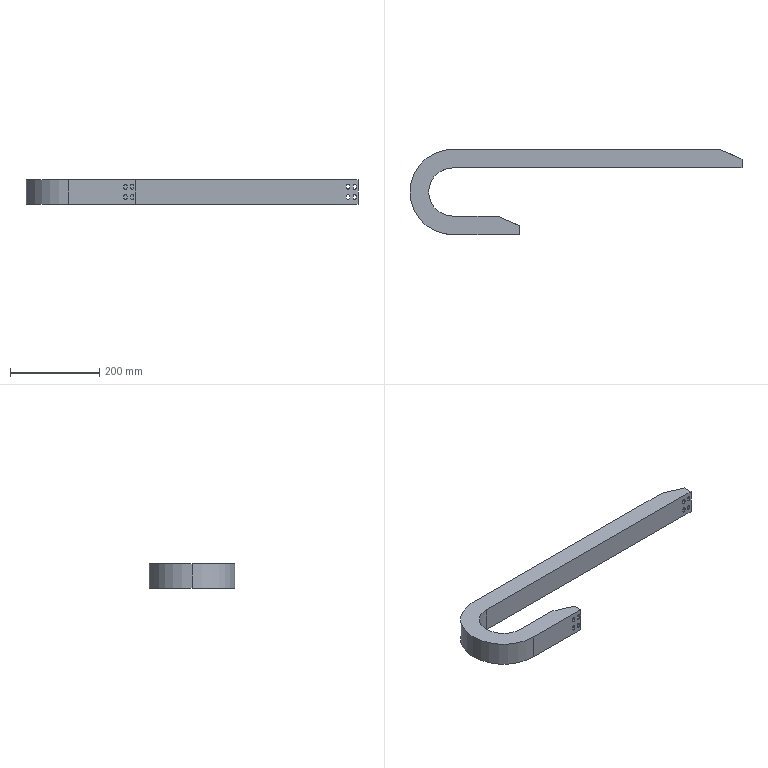Part | STEP file | P-0171514 modified_default | 1 solid | 64 faces | box 746 x 192 x 55 mm | volume 1359161 mm3 | cylinder 32 | plane 32 | commonest cylinder face diameters 7 x24 108 x2 125 x2 175 x2 192 x2